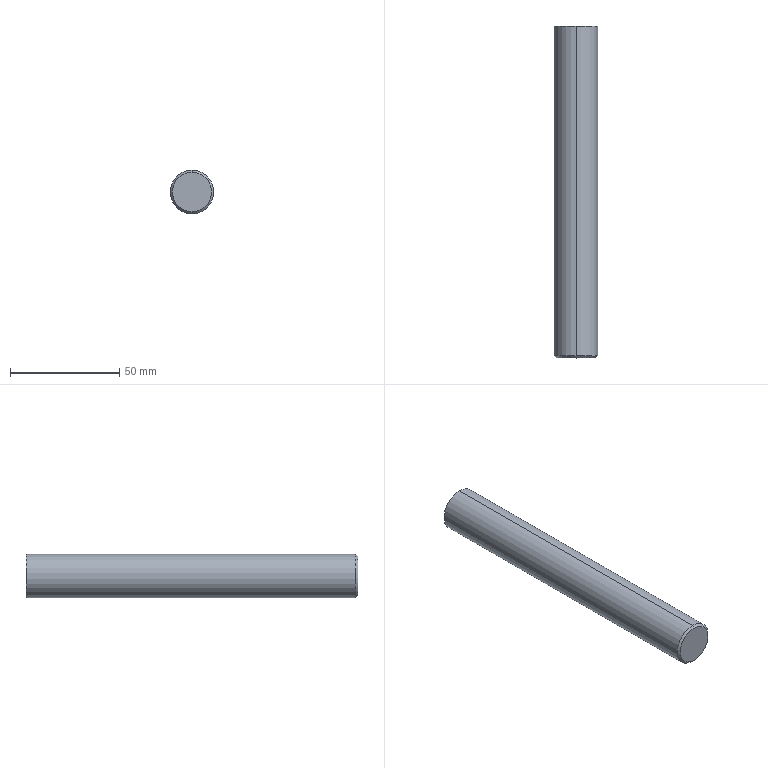Part | SolidWorks | features Chamfer 1, Extrusion 1 | 1 solid | 6 faces | box 20 x 152 x 20 mm | volume 47722 mm3 | cone 2 | cylinder 2 | plane 2 | commonest cylinder face diameters 20 x2
STEP:
#1=CARTESIAN_POINT('',(0.,-76.,-9.));
#2=VERTEX_POINT('',#1);
#3=CARTESIAN_POINT('',(0.,-76.,9.));
#4=VERTEX_POINT('',#3);
#5=CARTESIAN_POINT('',(0.,-76.,0.));
#6=DIRECTION('',(0.,-1.,0.));
#7=DIRECTION('',(0.,0.,1.));
#8=AXIS2_PLACEMENT_3D('',#5,#6,#7);
#9=CIRCLE('',#8,9.);
#10=EDGE_CURVE('',#2,#4,#9,.T.);
#11=ORIENTED_EDGE('',*,*,#10,.F.);
#12=CARTESIAN_POINT('',(0.,-75.,-10.));
#13=VERTEX_POINT('',#12);
#14=CARTESIAN_POINT('',(0.,-75.,-10.));
#15=DIRECTION('',(0.,0.7071,-0.7071));
#16=VECTOR('',#15,1000.);
#17=LINE('',#14,#16);
#18=EDGE_CURVE('',#2,#13,#17,.T.);
#19=ORIENTED_EDGE('',*,*,#18,.T.);
#20=CARTESIAN_POINT('',(0.,-75.,10.));
#21=VERTEX_POINT('',#20);
#22=CARTESIAN_POINT('',(0.,-75.,0.));
#23=DIRECTION('',(0.,1.,0.));
#24=DIRECTION('',(0.,0.,1.));
#25=AXIS2_PLACEMENT_3D('',#22,#23,#24);
#26=CIRCLE('',#25,10.);
#27=EDGE_CURVE('',#21,#13,#26,.T.);
#28=ORIENTED_EDGE('',*,*,#27,.F.);
#29=CARTESIAN_POINT('',(0.,-75.,10.));
#30=DIRECTION('',(0.,0.7071,0.7071));
#31=VECTOR('',#30,1000.);
#32=LINE('',#29,#31);
#33=EDGE_CURVE('',#4,#21,#32,.T.);
#34=ORIENTED_EDGE('',*,*,#33,.F.);
#35=EDGE_LOOP('',(#11,#19,#28,#34));
#36=FACE_OUTER_BOUND('',#35,.T.);
#37=CARTESIAN_POINT('',(0.,-75.,0.));
#38=DIRECTION('',(0.,1.,0.));
#39=DIRECTION('',(0.,0.,1.));
#40=AXIS2_PLACEMENT_3D('',#37,#38,#39);
#41=CONICAL_SURFACE('',#40,10.,0.7854);
#42=ADVANCED_FACE('',(#36),#41,.T.);
#43=CARTESIAN_POINT('',(0.,76.,10.));
#44=VERTEX_POINT('',#43);
#45=CARTESIAN_POINT('',(0.,76.,-10.));
#46=VERTEX_POINT('',#45);
#47=CARTESIAN_POINT('',(0.,76.,0.));
#48=DIRECTION('',(0.,1.,0.));
#49=DIRECTION('',(0.,0.,1.));
#50=AXIS2_PLACEMENT_3D('',#47,#48,#49);
#51=CIRCLE('',#50,10.);
#52=EDGE_CURVE('',#44,#46,#51,.T.);
#53=ORIENTED_EDGE('',*,*,#52,.F.);
#54=CARTESIAN_POINT('',(0.,76.,10.));
#55=DIRECTION('',(0.,-1.,0.));
#56=VECTOR('',#55,1000.);
#57=LINE('',#54,#56);
#58=EDGE_CURVE('',#44,#21,#57,.T.);
#59=ORIENTED_EDGE('',*,*,#58,.T.);
#60=ORIENTED_EDGE('',*,*,#27,.T.);
#61=CARTESIAN_POINT('',(0.,76.,-10.));
#62=DIRECTION('',(0.,-1.,0.));
#63=VECTOR('',#62,1000.);
#64=LINE('',#61,#63);
#65=EDGE_CURVE('',#46,#13,#64,.T.);
#66=ORIENTED_EDGE('',*,*,#65,.F.);
#67=EDGE_LOOP('',(#53,#59,#60,#66));
#68=FACE_OUTER_BOUND('',#67,.T.);
#69=CARTESIAN_POINT('',(0.,76.,0.));
#70=DIRECTION('',(0.,-1.,0.));
#71=DIRECTION('',(0.,0.,-1.));
#72=AXIS2_PLACEMENT_3D('',#69,#70,#71);
#73=CYLINDRICAL_SURFACE('',#72,10.);
#74=ADVANCED_FACE('',(#68),#73,.T.);
#75=ORIENTED_EDGE('',*,*,#58,.F.);
#76=CARTESIAN_POINT('',(0.,76.,0.));
#77=DIRECTION('',(0.,1.,0.));
#78=DIRECTION('',(0.,0.,1.));
#79=AXIS2_PLACEMENT_3D('',#76,#77,#78);
#80=CIRCLE('',#79,10.);
#81=EDGE_CURVE('',#46,#44,#80,.T.);
#82=ORIENTED_EDGE('',*,*,#81,.F.);
#83=ORIENTED_EDGE('',*,*,#65,.T.);
#84=CARTESIAN_POINT('',(0.,-75.,0.));
#85=DIRECTION('',(0.,1.,0.));
#86=DIRECTION('',(0.,0.,1.));
#87=AXIS2_PLACEMENT_3D('',#84,#85,#86);
#88=CIRCLE('',#87,10.);
#89=EDGE_CURVE('',#13,#21,#88,.T.);
#90=ORIENTED_EDGE('',*,*,#89,.T.);
#91=EDGE_LOOP('',(#75,#82,#83,#90));
#92=FACE_OUTER_BOUND('',#91,.T.);
#93=CARTESIAN_POINT('',(0.,76.,0.));
#94=DIRECTION('',(0.,-1.,0.));
#95=DIRECTION('',(0.,0.,-1.));
#96=AXIS2_PLACEMENT_3D('',#93,#94,#95);
#97=CYLINDRICAL_SURFACE('',#96,10.);
#98=ADVANCED_FACE('',(#92),#97,.T.);
#99=ORIENTED_EDGE('',*,*,#81,.T.);
#100=ORIENTED_EDGE('',*,*,#52,.T.);
#101=EDGE_LOOP('',(#99,#100));
#102=FACE_OUTER_BOUND('',#101,.T.);
#103=CARTESIAN_POINT('',(0.,76.,0.));
#104=DIRECTION('',(0.,1.,0.));
#105=DIRECTION('',(0.,0.,1.));
#106=AXIS2_PLACEMENT_3D('',#103,#104,#105);
#107=PLANE('',#106);
#108=ADVANCED_FACE('',(#102),#107,.T.);
#109=CARTESIAN_POINT('',(0.,-76.,0.));
#110=DIRECTION('',(0.,-1.,0.));
#111=DIRECTION('',(0.,0.,1.));
#112=AXIS2_PLACEMENT_3D('',#109,#110,#111);
#113=CIRCLE('',#112,9.);
#114=EDGE_CURVE('',#4,#2,#113,.T.);
#115=ORIENTED_EDGE('',*,*,#114,.T.);
#116=ORIENTED_EDGE('',*,*,#10,.T.);
#117=EDGE_LOOP('',(#115,#116));
#118=FACE_OUTER_BOUND('',#117,.T.);
#119=CARTESIAN_POINT('',(0.,-76.,0.));
#120=DIRECTION('',(0.,1.,0.));
#121=DIRECTION('',(0.,0.,1.));
#122=AXIS2_PLACEMENT_3D('',#119,#120,#121);
#123=PLANE('',#122);
#124=ADVANCED_FACE('',(#118),#123,.F.);
#125=ORIENTED_EDGE('',*,*,#18,.F.);
#126=ORIENTED_EDGE('',*,*,#114,.F.);
#127=ORIENTED_EDGE('',*,*,#33,.T.);
#128=ORIENTED_EDGE('',*,*,#89,.F.);
#129=EDGE_LOOP('',(#125,#126,#127,#128));
#130=FACE_OUTER_BOUND('',#129,.T.);
#131=CARTESIAN_POINT('',(0.,-75.,0.));
#132=DIRECTION('',(0.,1.,0.));
#133=DIRECTION('',(0.,0.,1.));
#134=AXIS2_PLACEMENT_3D('',#131,#132,#133);
#135=CONICAL_SURFACE('',#134,10.,0.7854);
#136=ADVANCED_FACE('',(#130),#135,.T.);
#137=CLOSED_SHELL('',(#42,#74,#98,#108,#124,#136));
#138=MANIFOLD_SOLID_BREP('',#137);
#139=CARTESIAN_POINT('',(0.,0.,0.));
#140=DIRECTION('',(0.,0.,1.));
#141=DIRECTION('',(1.,0.,0.));
#142=AXIS2_PLACEMENT_3D('',#139,#140,#141);
#143=(LENGTH_UNIT()NAMED_UNIT(*)SI_UNIT(.MILLI.,.METRE.));
#144=UNCERTAINTY_MEASURE_WITH_UNIT(LENGTH_MEASURE(0.00001),#143,'','');
#145=(NAMED_UNIT(*)PLANE_ANGLE_UNIT()SI_UNIT($,.RADIAN.));
#146=(NAMED_UNIT(*)SI_UNIT($,.STERADIAN.)SOLID_ANGLE_UNIT());
#147=(GEOMETRIC_REPRESENTATION_CONTEXT(3)GLOBAL_UNCERTAINTY_ASSIGNED_CONTEXT((#144))GLOBAL_UNIT_ASSIGNED_CONTEXT((#143,#145,#146))REPRESENTATION_CONTEXT('',''));
#148=ADVANCED_BREP_SHAPE_REPRESENTATION('',(#138,#142),#147);